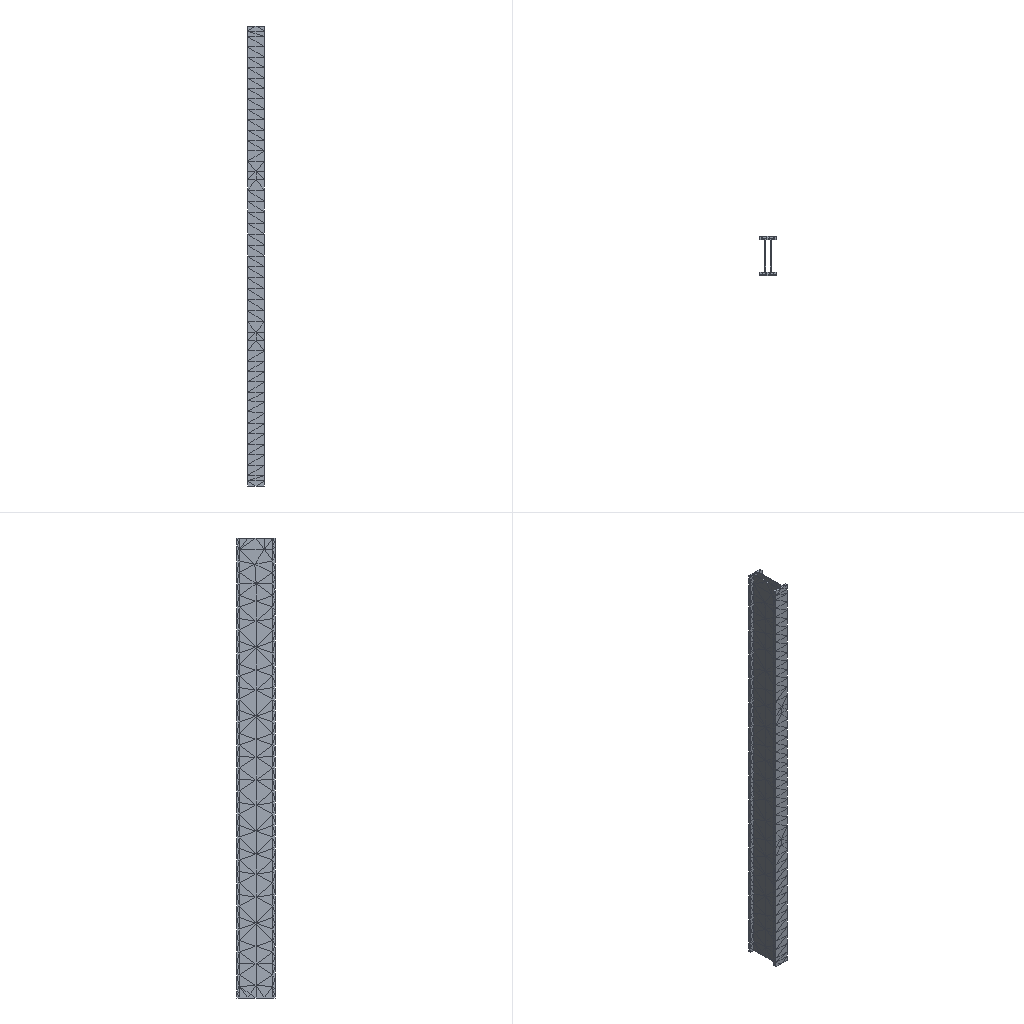Simulation study | ansys workbench
Set-up summary:
category,name,step,type,value,unit,region
solver,ansys_workbench
units,mm-N-s-tonne (MPa),,stated,"/units,MPA"
analysis,LS1,,static
load_step,LS1,LS1,static,nsubst=1; time=1
mesh,nodes,,,5493
mesh,elements,,,2887
element_type,SOLID187,,,2887
material,Beam,,E,206000,tonne s^-2 mm^-1
material,Beam,,nu,0.28
load,,LS1,pressure,-245000 [n=6],,all
bc,Fixed Supports,model,fixed,[dofs=ALL],,_FIXEDSU
bc,Constant Zero Displacement X,model,fixed,[dofs=UX],,_DISPZEROUX
named_set,_FIXEDSU,,node,30
named_set,_DISPZEROUX,,node,180
Ansys APDL input file, long lists of numbers shortened:
/batch
/config,noeldb,1     ! force off writing results to database
*get,_wallstrt,active,,time,wall
! ANSYS input file written by Workbench version 2021 R1
! File used for geometry attach:
/title,wbnew--____ (B5)
! ****** Begin Custom Load Command Snippet ******
/COM, ACT Extensions:
/COM,     LSDYNA, 2021.1
/COM,
! ****** End   Custom Load Command Snippet ******
*DIM,_wb_ProjectScratch_dir,string,248
_wb_ProjectScratch_dir(1) = ''
*DIM,_wb_SolverFiles_dir,string,248
_wb_SolverFiles_dir(1) = ''
*DIM,_wb_userfiles_dir,string,248
_wb_userfiles_dir(1) = ''
/com,--- Data in consistent NMM units. See Solving Units in the help system for more information.
/units,MPA
/nopr
/wb,file,start              !  signify a WB generated input file
/prep7
! Turn off shape checking because checks already performed inside WB mesher.
! See help system for more information.
SHPP,OFF,,NOWARN
/nolist
etcon,set             ! allow ANSYS to choose best KEYOP's for 180x elements, resets any applicable keyopt to MAPDL defaults
/com,*********** Nodes for the whole assembly ***********
nblock,3,,6042
(1i9,3e20.9e3)
        1    -4.500000000E+01    -2.885684759E+01     0.000000000E+00
! (5492 more lines like these left out)
-1
/wb,elem,start            !  set before creation of elements
/com,*********** Elements for Body 1 "1" ***********
et,1,187
eblock,19,solid,,2887
(19i9)
        1        1        1        1        0        0        0        0       10        0        1      101      108      378      472     1945     2008     1948     1951
! (5773 more lines like these left out)
-1
/wb,elem,end               !  done creating elements
/com,*********** Send User Defined Coordinate System(s) ***********
csys,0
toffst,273.15,  ! Temperature offset from absolute zero
/com,*********** Set Reference Temperature ***********
tref,22.
/wb,mat,start              !  starting to send materials
/com,*********** Send Materials ***********
MP,EX,1,206000,	! tonne s^-2 mm^-1
MP,NUXY,1,0.28,
/wb,mat,end                !  done sending materials
!************************* Model Summary ********************
!1,	Beam,	matid,	1
!************************* End Model Summary ********************
! get the diagonal of the bounding box. Needed later for other things
*get,_xmin,node,,mnloc,x
*get,_ymin,node,,mnloc,y
*get,_zmin,node,,mnloc,z
*get,_xmax,node,,mxloc,x
*get,_ymax,node,,mxloc,y
*get,_zmax,node,,mxloc,z
_ASMDIAG=(_xmax-_xmin)*(_xmax-_xmin)+(_ymax-_ymin)*(_ymax-_ymin)+(_zmax-_zmin)*(_zmax-_zmin)
_ASMDIAG=SQRT(_ASMDIAG)
/wb,contact,start          !  starting to send contact
/wb,contact,end            !  done creating contacts
/golist
/wb,load,start             !  starting to send loads
/com,*********** Fixed Supports ***********
CMBLOCK,_FIXEDSU,NODE,       30
(8i10)
        66        67        68        75        82        83        98        99
       428       436       444       462      1637      1640      1642      1645
      1648      1650      1653      1657      1725      1728      1794      1800
      1929      1930      1936      1937      4395      4430
cmsel,s,_FIXEDSU
d,all,all
nsel,all
/com,******* Constant Zero Displacement X *******
CMBLOCK,_DISPZEROUX,NODE,      180
(8i10)
         1         2         3        23        43        44        45        46
! (22 more lines like these left out)
cmsel,s,_DISPZEROUX
d,all,ux,0
nsel,all
/com,*********** Define Vertex Force Using Follower Elements ***********
et,2,201
keyo,2,1,1           ! Keep the direction constant
keyo,2,2,1           ! Apply Forces only, not moment
mat,2
real,2
type,2
en,4504,353
r,2
rmod,2,1,1.0,              ! FX
mat,3
real,3
type,2
en,4505,353
r,3
rmod,3,2,1.0,              ! FY
mat,4
real,4
type,2
en,4506,353
r,4
rmod,4,3,1.0,              ! FZ
/com,*********** Define Vertex Force Using Follower Elements ***********
et,5,201
keyo,5,1,1           ! Keep the direction constant
keyo,5,2,1           ! Apply Forces only, not moment
mat,5
real,5
type,5
en,4507,355
r,5
rmod,5,1,1.0,              ! FX
mat,6
real,6
type,5
en,4508,355
r,6
rmod,6,2,1.0,              ! FY
mat,7
real,7
type,5
en,4509,355
r,7
rmod,7,3,1.0,              ! FZ
/com,*********** Define Vertex Force Using Follower Elements ***********
et,8,201
keyo,8,1,1           ! Keep the direction constant
keyo,8,2,1           ! Apply Forces only, not moment
mat,8
real,8
type,8
en,4510,357
r,8
rmod,8,1,1.0,              ! FX
mat,9
real,9
type,8
en,4511,357
r,9
rmod,9,2,1.0,              ! FY
mat,10
real,10
type,8
en,4512,357
r,10
rmod,10,3,1.0,              ! FZ
/com,*********** Define Vertex Force Using Follower Elements ***********
et,11,201
keyo,11,1,1           ! Keep the direction constant
keyo,11,2,1           ! Apply Forces only, not moment
mat,11
real,11
type,11
en,4513,359
r,11
rmod,11,1,1.0,              ! FX
mat,12
real,12
type,11
en,4514,359
r,12
rmod,12,2,1.0,              ! FY
mat,13
real,13
type,11
en,4515,359
r,13
rmod,13,3,1.0,              ! FZ
/com,*********** Define Vertex Force Using Follower Elements ***********
et,14,201
keyo,14,1,1           ! Keep the direction constant
keyo,14,2,1           ! Apply Forces only, not moment
mat,14
real,14
type,14
en,4516,361
r,14
rmod,14,1,1.0,              ! FX
mat,15
real,15
type,14
en,4517,361
r,15
rmod,15,2,1.0,              ! FY
mat,16
real,16
type,14
en,4518,361
r,16
rmod,16,3,1.0,              ! FZ
/com,*********** Define Vertex Force Using Follower Elements ***********
et,17,201
keyo,17,1,1           ! Keep the direction constant
keyo,17,2,1           ! Apply Forces only, not moment
mat,17
real,17
type,17
en,4519,363
r,17
rmod,17,1,1.0,              ! FX
mat,18
real,18
type,17
en,4520,363
r,18
rmod,18,2,1.0,              ! FY
mat,19
real,19
type,17
en,4521,363
r,19
rmod,19,3,1.0,              ! FZ
/gst,on,on
fini
*get,_numnode,node,0,count
*get,_numelem,elem,0,count
*get, _MAXELEMNUM, elem, 0, NUM, MAX
*get, _MAXNODENUM, node, 0, NUM, MAX
*get, _MAXELEMTYPE, etyp, 0, NUM, MAX
*get, _MAXREALCONST, real, 0, NUM, MAX
/go
/wb,load,end               !  done creating loads
/com,--- Number of total nodes = %_numnode%
/com,--- Number of contact elements = 0
/com,--- Number of spring elements = 0
/com,--- Number of bearing elements = 0
/com,--- Number of solid elements = 2887
/com,--- Number of condensed parts = 0
/com,--- Number of total elements = %_numelem%
*get,_wallbsol,active,,time,wall
/com,****************************************************************************
/com,*************************    SOLUTION       ********************************
/com,****************************************************************************
/solu
antype,0                   ! static analysis
_thickRatio=  0     ! Ratio of thick parts in the model
eqsl,sparse,,,,,1
cntr,print,1               ! print out contact info and also make no initial contact an error
dmpoption,emat,no             ! Don't combine emat file for DANSYS
dmpoption,esav,no             ! Don't combine esav file for DANSYS
nldiag,cont,iter           ! print out contact info each equilibrium iteration
rescontrol,,none                 ! Do not keep any restart files
/com,****************************************************
/com,******************* SOLVE FOR LS 1 OF 1 ****************
esel,s,real,,2
sfe,all,1,pres,1,0.
esel,s,real,,3
sfe,all,1,pres,1,-245000.
esel,s,real,,4
sfe,all,1,pres,1,0.
esel,s,real,,5
sfe,all,1,pres,1,0.
esel,s,real,,6
sfe,all,1,pres,1,-245000.
esel,s,real,,7
sfe,all,1,pres,1,0.
esel,s,real,,8
sfe,all,1,pres,1,0.
esel,s,real,,9
sfe,all,1,pres,1,-245000.
esel,s,real,,10
sfe,all,1,pres,1,0.
esel,s,real,,11
sfe,all,1,pres,1,0.
esel,s,real,,12
sfe,all,1,pres,1,-245000.
esel,s,real,,13
sfe,all,1,pres,1,0.
esel,s,real,,14
sfe,all,1,pres,1,0.
esel,s,real,,15
sfe,all,1,pres,1,-245000.
esel,s,real,,16
sfe,all,1,pres,1,0.
esel,s,real,,17
sfe,all,1,pres,1,0.
esel,s,real,,18
sfe,all,1,pres,1,-245000.
esel,s,real,,19
sfe,all,1,pres,1,0.
esel,all
/nopr
/gopr
/nolist
nsub,1,1,1
time,1.
outres,erase
outres,all,none
outres,nsol,all,
outres,rsol,all
outres,eangl,all
outres,etmp,all
outres,veng,all
outres,strs,all,
outres,epel,all,
outres,eppl,all,
outres,cont,all,
! *********** WB SOLVE COMMAND ***********
! check interactive state
*get,ANSINTER_,active,,int
*if,ANSINTER_,ne,0,then
/eof
*endif
solve
/com *************** Write FE CONNECTORS *********
CEWRITE,file,ce,,INTE
/com,****************************************************
/com,*************** FINISHED SOLVE FOR LS 1 *************
*get,_wallasol,active,,time,wall
/nopr
*get,_numnode,node,0,count
*get,_numelem,elem,0,count
*get, _MAXELEMNUM, elem, 0, NUM, MAX
*get, _MAXNODENUM, node, 0, NUM, MAX,,,INTERNAL
*get, _MAXELEMTYPE, etyp, 0, NUM, MAX
*get, _MAXREALCONST, real, 0, NUM, MAX
/gopr
/post1
xmlo,ENCODING,ISO-8859-1
xmlo,parm
/xml,parm,xml
fini
/gopr
*get,_walldone,active,,time,wall
_preptime=(_wallbsol-_wallstrt)*3600
_solvtime=(_wallasol-_wallbsol)*3600
_posttime=(_walldone-_wallasol)*3600
_totaltim=(_walldone-_wallstrt)*3600
*get,_dlbratio,active,0,solu,dlbr
*get,_combtime,active,0,solu,comb
/com,--- Total number of nodes = %_numnode%
/com,--- Total number of elements = %_numelem%
/com,--- Element load balance ratio = %_dlbratio%
/com,--- Time to combine distributed files = %_combtime%
/wb,file,end               ! done with WB generated input
Results summary:
result,analyses[0].index,,,1
result,analyses[0].system,,,SYS-1
result,analyses[0].deck,,,deck.dat
result,analyses[0].solve_status,,,completed
result,analyses[0].analysis_type,,,static
result,analyses[0].physics,,,mechanical
result,analyses[0].unit_system,,,"NMM: mm, ton, N, s, mV, mA, degC"
result,analyses[0].n_sets,,,1
result,analyses[0].load_steps[0].set,set=1,,1
result,analyses[0].load_steps[0].time_or_freq,set=1,,1
result,analyses[0].load_steps[0].max_displacement_magnitude,set=1,,2.601
result,analyses[0].load_steps[0].max_von_mises_nodal,set=1,,55.706
result,analyses[0].load_steps[0].reaction_force_sum_xyz[1],set=1,,-8.0719e-05
result,analyses[0].load_steps[0].reaction_force_sum_xyz[2],set=1,,1.47e+06
result,analyses[0].load_steps[0].reaction_force_sum_xyz[3],set=1,,-8.57713e-06
result,geometry_export[0][0],,,.step
result,geometry_export[0][1],,,ok
result,geometry_export[0][2],,,1